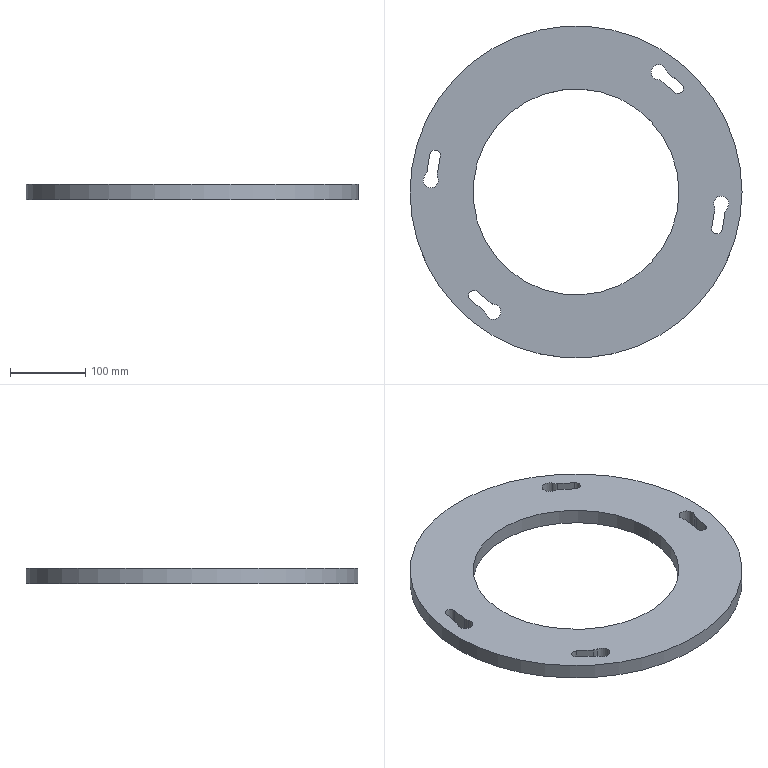CAM job | NX | 3-axis milling | part box 440 x 440 x 20 mm | stock box 440 x 440 x 20 mm
Tools:
number,name,description,diameter,corner_radius,flute_length,length,flutes
10,D10,Milling Tool-5 Parameters,10.0,0.0,50.0,75.0,2
9,D10JING,Milling Tool-5 Parameters,10.0,0.0,50.0,75.0,2
7,D6A45,Milling Tool-5 Parameters,6.0,0.0,3.0,3.0,2
Operations:
program,operation,operation_type,tool,method,geometry_group,spindle_rpm,surface_speed,feed_per_tooth,feed_cut,feed_plunge,cut_length_mm,path_length_mm,cut_time_min,machine_time_min
1,ZLEVEL_PROFILE_COPY_1,ZLevelMilling,D10,METHOD,A,2200.0,69.0,0.5,2200.0,100.0,32733.023,34176.396,14.879,15.023
1,ZLEVEL_PROFILE_COPY,ZLevelMilling,D10JING,METHOD,A,5000.0,157.0,0.12,1200.0,100.0,398.886,1894.83,0.3324,0.482
1,ZLEVEL_PROFILE_COPY_COPY,ZLevelMilling,D6A45,METHOD,A,7500.0,141.0,0.08,1200.0,100.0,501.224,2254.718,0.4177,0.593